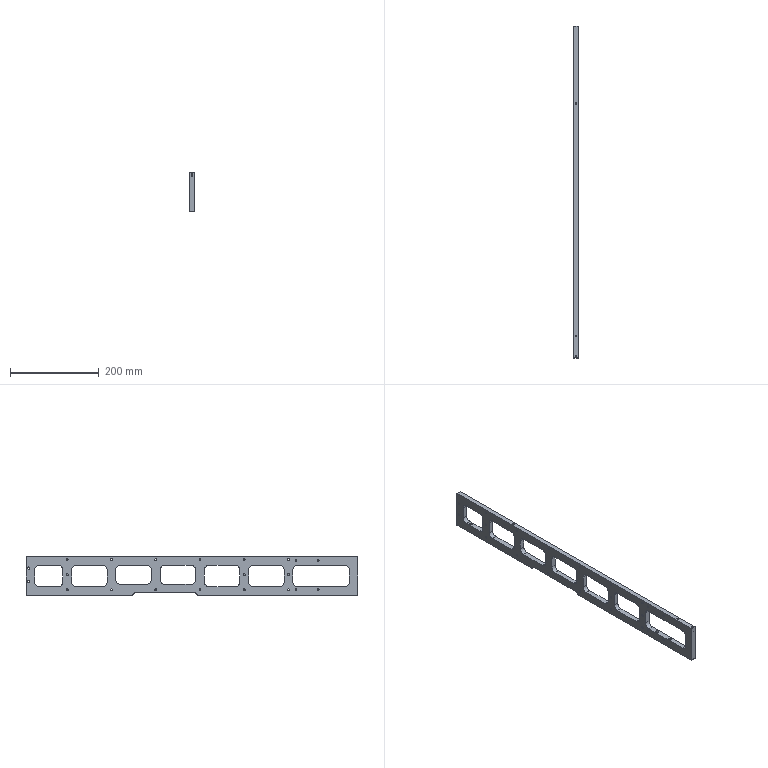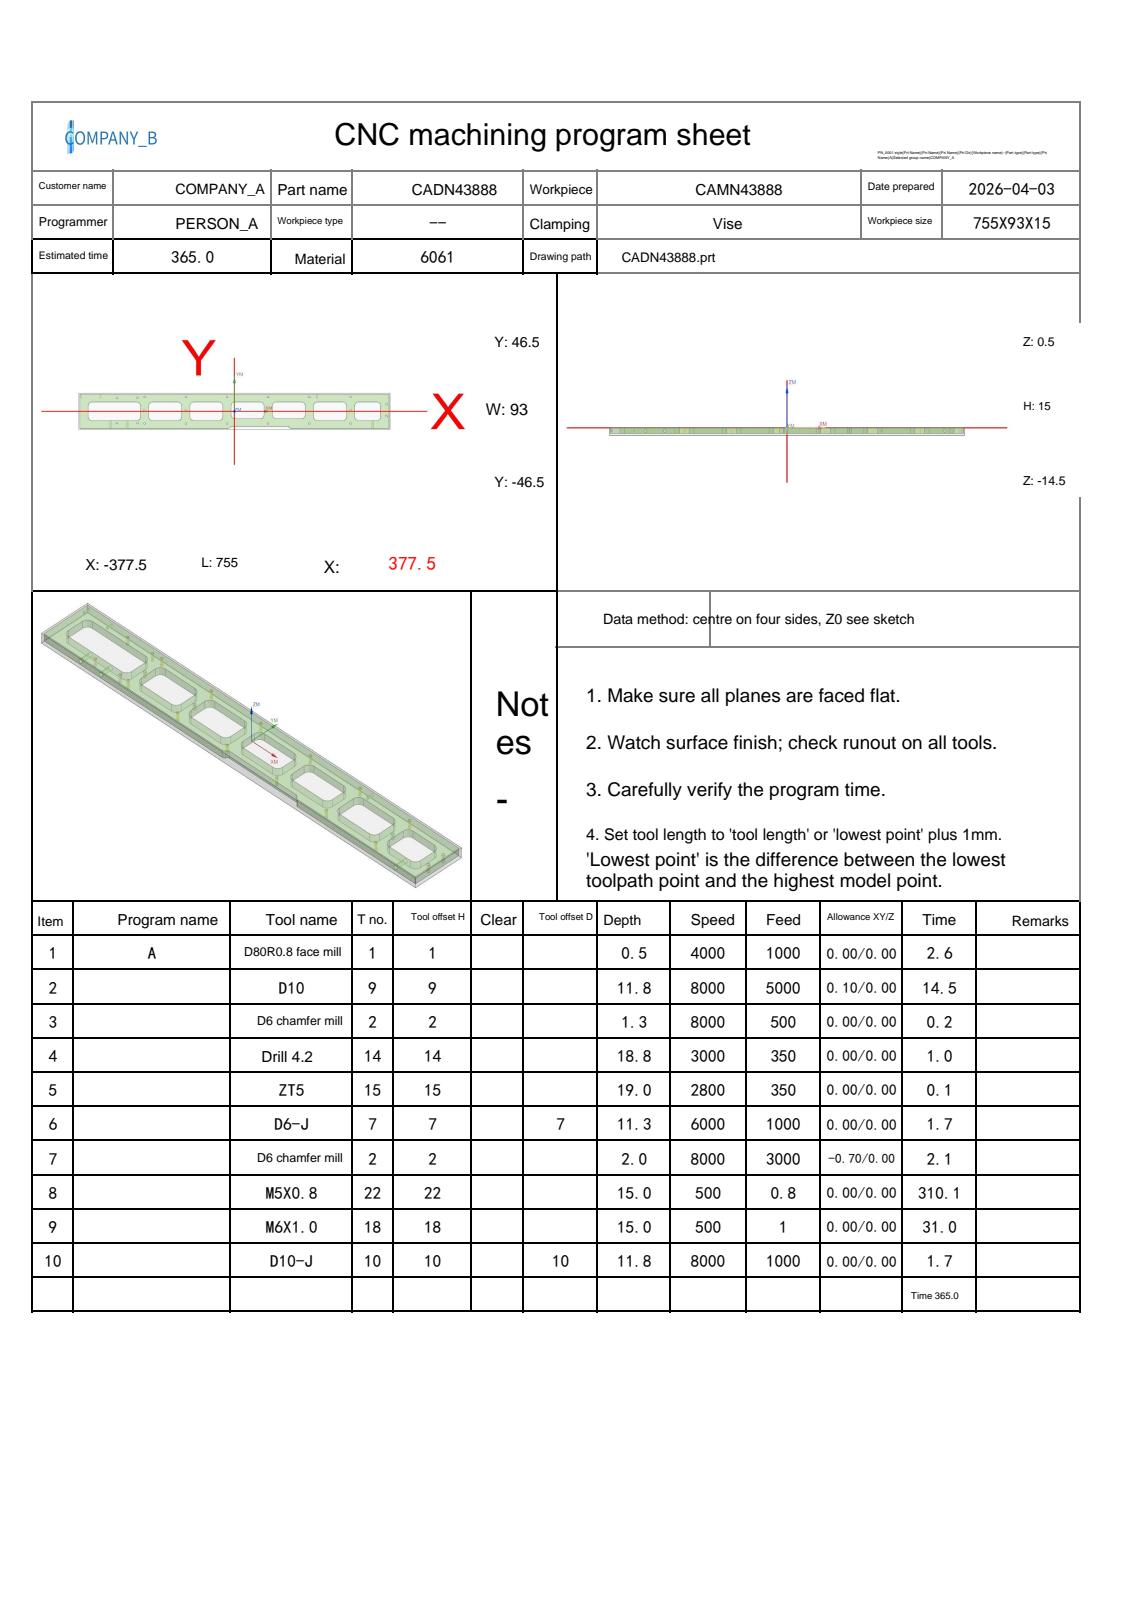NC program | NX | posted by the shop | part box 11 x 750 x 88 mm
Lines 1862 to 2351 of 2351:
N7 T02 M06
(D6 chamfer mill  D=6. R=0. H=02 ce=0.00 di=0.00)
G00 G90 G54 X-.25 Y45.828 M03 S8000
G43 H02 Z20.
M08
Z2.399
G01 Z-1.5 F3000.
G03 X-.33 Y45.528 I.52 J-.3
X-.03 Y45.008 I.6 J0.0
G01 X0.0 Y45.
X374.
G02 X376. Y43. I0.0 J-2.
G01 Y-43.
G02 X374. Y-45. I-2. J0.0
G01 X137.165
G02 X131.666 Y-41.4 I0.0 J6.
G03 X128. Y-39. I-3.666 J-1.6
G01 X-6.
G03 X-9.666 Y-41.4 I0.0 J-4.
G02 X-15.165 Y-45. I-5.499 J2.4
G01 X-374.
G02 X-376. Y-43. I0.0 J2.
G01 Y43.
G02 X-374. Y45. I2. J0.0
G01 X0.0
X.03 Y45.008
G03 X.33 Y45.528 I-.3 J.52
X.25 Y45.828 I-.6 J0.0
G01 Z2.399
G00 Z20.
X323.25 Y-22.172
Z2.399
G01 Z-1.5
G03 X323.17 Y-22.472 I.52 J-.3
X323.47 Y-22.992 I.6 J0.0
G01 X323.5 Y-23.
X345.
G03 X354. Y-14. I0.0 J9.
G01 Y14.
G03 X345. Y23. I-9. J0.0
G01 X302.
G03 X293. Y14. I0.0 J-9.
G01 Y-14.
G03 X302. Y-23. I9. J0.0
G01 X323.5
X323.53 Y-22.992
G03 X323.83 Y-22.472 I-.3 J.52
X323.75 Y-22.172 I-.6 J0.0
G01 Z2.399
G00 Z20.
X231.75
Z2.399
G01 Z-1.5
G03 X231.67 Y-22.472 I.52 J-.3
X231.97 Y-22.992 I.6 J0.0
G01 X232. Y-23.
X262.
G03 X271. Y-14. I0.0 J9.
G01 Y14.
G03 X262. Y23. I-9. J0.0
G01 X202.
G03 X193. Y14. I0.0 J-9.
G01 Y-14.
G03 X202. Y-23. I9. J0.0
G01 X232.
X232.03 Y-22.992
G03 X232.33 Y-22.472 I-.3 J.52
X232.25 Y-22.172 I-.6 J0.0
G01 Z2.399
G00 Z20.
X131.75 Y-17.172
Z2.399
G01 Z-1.5
G03 X131.67 Y-17.472 I.52 J-.3
X131.97 Y-17.992 I.6 J0.0
G01 X132. Y-18.
X162.
G03 X171. Y-9. I0.0 J9.
G01 Y14.
G03 X162. Y23. I-9. J0.0
G01 X102.
G03 X93. Y14. I0.0 J-9.
G01 Y-9.
G03 X102. Y-18. I9. J0.0
G01 X132.
X132.03 Y-17.992
G03 X132.33 Y-17.472 I-.3 J.52
X132.25 Y-17.172 I-.6 J0.0
G01 Z2.399
G00 Z20.
X31.75
Z2.399
G01 Z-1.5
G03 X31.67 Y-17.472 I.52 J-.3
X31.97 Y-17.992 I.6 J0.0
G01 X32. Y-18.
X62.
G03 X71. Y-9. I0.0 J9.
G01 Y14.
G03 X62. Y23. I-9. J0.0
G01 X2.
G03 X-7. Y14. I0.0 J-9.
G01 Y-9.
G03 X2. Y-18. I9. J0.0
G01 X32.
X32.03 Y-17.992
G03 X32.33 Y-17.472 I-.3 J.52
X32.25 Y-17.172 I-.6 J0.0
G01 Z2.399
G00 Z20.
X-68.25 Y-22.172
Z2.399
G01 Z-1.5
G03 X-68.33 Y-22.472 I.52 J-.3
X-68.03 Y-22.992 I.6 J0.0
G01 X-68. Y-23.
X-38.
G03 X-29. Y-14. I0.0 J9.
G01 Y14.
G03 X-38. Y23. I-9. J0.0
G01 X-98.
G03 X-107. Y14. I0.0 J-9.
G01 Y-14.
G03 X-98. Y-23. I9. J0.0
G01 X-68.
X-67.97 Y-22.992
G03 X-67.67 Y-22.472 I-.3 J.52
X-67.75 Y-22.172 I-.6 J0.0
G01 Z2.399
G00 Z20.
X-168.25
Z2.399
G01 Z-1.5
G03 X-168.33 Y-22.472 I.52 J-.3
X-168.03 Y-22.992 I.6 J0.0
G01 X-168. Y-23.
X-138.
G03 X-129. Y-14. I0.0 J9.
G01 Y14.
G03 X-138. Y23. I-9. J0.0
G01 X-198.
G03 X-207. Y14. I0.0 J-9.
G01 Y-14.
G03 X-198. Y-23. I9. J0.0
G01 X-168.
X-167.97 Y-22.992
G03 X-167.67 Y-22.472 I-.3 J.52
X-167.75 Y-22.172 I-.6 J0.0
G01 Z2.399
G00 Z20.
X-291.75
Z2.399
G01 Z-1.5
G03 X-291.83 Y-22.472 I.52 J-.3
X-291.53 Y-22.992 I.6 J0.0
G01 X-291.5 Y-23.
X-238.
G03 X-229. Y-14. I0.0 J9.
G01 Y14.
G03 X-238. Y23. I-9. J0.0
G01 X-345.
G03 X-354. Y14. I0.0 J-9.
G01 Y-14.
G03 X-345. Y-23. I9. J0.0
G01 X-291.5
X-291.47 Y-22.992
G03 X-291.17 Y-22.472 I-.3 J.52
X-291.25 Y-22.172 I-.6 J0.0
G01 Z2.399
G00 Z20.
G00 G90 X282.694 Y37.093 M03 S8000
Z20.
Z-.5
G01 Z-1. F500.
X283.5 Y37.2
G03 X282. Y38.7 I-1.5 J0.0
X280.3 Y37. I0.0 J-1.7
X282. Y35.3 I1.7 J0.0
X283.7 Y37. I0.0 J1.7
X282. Y38.7 I-1.7 J0.0
X280.5 Y37.2 I0.0 J-1.5
G01 X281.306 Y37.093
Z-.5
G00 Z20.
X282.694 Y-30.907
Z-.5
G01 Z-1.
X283.5 Y-30.8
G03 X282. Y-29.3 I-1.5 J0.0
X280.3 Y-31. I0.0 J-1.7
X282. Y-32.7 I1.7 J0.0
X283.7 Y-31. I0.0 J1.7
X282. Y-29.3 I-1.7 J0.0
X280.5 Y-30.8 I0.0 J-1.5
G01 X281.306 Y-30.907
Z-.5
G00 Z20.
X182.694
Z-.5
G01 Z-1.
X183.5 Y-30.8
G03 X182. Y-29.3 I-1.5 J0.0
X180.3 Y-31. I0.0 J-1.7
X182. Y-32.7 I1.7 J0.0
X183.7 Y-31. I0.0 J1.7
X182. Y-29.3 I-1.7 J0.0
X180.5 Y-30.8 I0.0 J-1.5
G01 X181.306 Y-30.907
Z-.5
G00 Z20.
X182.694 Y37.093
Z-.5
G01 Z-1.
X183.5 Y37.2
G03 X182. Y38.7 I-1.5 J0.0
X180.3 Y37. I0.0 J-1.7
X182. Y35.3 I1.7 J0.0
X183.7 Y37. I0.0 J1.7
X182. Y38.7 I-1.7 J0.0
X180.5 Y37.2 I0.0 J-1.5
G01 X181.306 Y37.093
Z-.5
G00 Z20.
X82.694
Z-.5
G01 Z-1.
X83.5 Y37.2
G03 X82. Y38.7 I-1.5 J0.0
X80.3 Y37. I0.0 J-1.7
X82. Y35.3 I1.7 J0.0
X83.7 Y37. I0.0 J1.7
X82. Y38.7 I-1.7 J0.0
X80.5 Y37.2 I0.0 J-1.5
G01 X81.306 Y37.093
Z-.5
G00 Z20.
X82.694 Y-30.907
Z-.5
G01 Z-1.
X83.5 Y-30.8
G03 X82. Y-29.3 I-1.5 J0.0
X80.3 Y-31. I0.0 J-1.7
X82. Y-32.7 I1.7 J0.0
X83.7 Y-31. I0.0 J1.7
X82. Y-29.3 I-1.7 J0.0
X80.5 Y-30.8 I0.0 J-1.5
G01 X81.306 Y-30.907
Z-.5
G00 Z20.
X-17.306
Z-.5
G01 Z-1.
X-16.5 Y-30.8
G03 X-18. Y-29.3 I-1.5 J0.0
X-19.7 Y-31. I0.0 J-1.7
X-18. Y-32.7 I1.7 J0.0
X-16.3 Y-31. I0.0 J1.7
X-18. Y-29.3 I-1.7 J0.0
X-19.5 Y-30.8 I0.0 J-1.5
G01 X-18.694 Y-30.907
Z-.5
G00 Z20.
X-17.306 Y37.093
Z-.5
G01 Z-1.
X-16.5 Y37.2
G03 X-18. Y38.7 I-1.5 J0.0
X-19.7 Y37. I0.0 J-1.7
X-18. Y35.3 I1.7 J0.0
X-16.3 Y37. I0.0 J1.7
X-18. Y38.7 I-1.7 J0.0
X-19.5 Y37.2 I0.0 J-1.5
G01 X-18.694 Y37.093
Z-.5
G00 Z20.
X-117.306
Z-.5
G01 Z-1.
X-116.5 Y37.2
G03 X-118. Y38.7 I-1.5 J0.0
X-119.7 Y37. I0.0 J-1.7
X-118. Y35.3 I1.7 J0.0
X-116.3 Y37. I0.0 J1.7
X-118. Y38.7 I-1.7 J0.0
X-119.5 Y37.2 I0.0 J-1.5
G01 X-118.694 Y37.093
Z-.5
G00 Z20.
X-117.306 Y-30.907
Z-.5
G01 Z-1.
X-116.5 Y-30.8
G03 X-118. Y-29.3 I-1.5 J0.0
X-119.7 Y-31. I0.0 J-1.7
X-118. Y-32.7 I1.7 J0.0
X-116.3 Y-31. I0.0 J1.7
X-118. Y-29.3 I-1.7 J0.0
X-119.5 Y-30.8 I0.0 J-1.5
G01 X-118.694 Y-30.907
Z-.5
G00 Z20.
X-217.306
Z-.5
G01 Z-1.
X-216.5 Y-30.8
G03 X-218. Y-29.3 I-1.5 J0.0
X-219.7 Y-31. I0.0 J-1.7
X-218. Y-32.7 I1.7 J0.0
X-216.3 Y-31. I0.0 J1.7
X-218. Y-29.3 I-1.7 J0.0
X-219.5 Y-30.8 I0.0 J-1.5
G01 X-218.694 Y-30.907
Z-.5
G00 Z20.
X-234.306 Y-30.157
Z-.5
G01 Z-1.
X-233.5 Y-30.05
G03 X-235. Y-28.55 I-1.5 J0.0
X-236.7 Y-30.25 I0.0 J-1.7
X-235. Y-31.95 I1.7 J0.0
X-233.3 Y-30.25 I0.0 J1.7
X-235. Y-28.55 I-1.7 J0.0
X-236.5 Y-30.05 I0.0 J-1.5
G01 X-235.694 Y-30.157
Z-.5
G00 Z20.
X-284.306
Z-.5
G01 Z-1.
X-283.5 Y-30.05
G03 X-285. Y-28.55 I-1.5 J0.0
X-286.7 Y-30.25 I0.0 J-1.7
X-285. Y-31.95 I1.7 J0.0
X-283.3 Y-30.25 I0.0 J1.7
X-285. Y-28.55 I-1.7 J0.0
X-286.5 Y-30.05 I0.0 J-1.5
G01 X-285.694 Y-30.157
Z-.5
G00 Z20.
X-284.306 Y35.343
Z-.5
G01 Z-1.
X-283.5 Y35.45
G03 X-285. Y36.95 I-1.5 J0.0
X-286.7 Y35.25 I0.0 J-1.7
X-285. Y33.55 I1.7 J0.0
X-283.3 Y35.25 I0.0 J1.7
X-285. Y36.95 I-1.7 J0.0
X-286.5 Y35.45 I0.0 J-1.5
G01 X-285.694 Y35.343
Z-.5
G00 Z20.
X-234.306
Z-.5
G01 Z-1.
X-233.5 Y35.45
G03 X-235. Y36.95 I-1.5 J0.0
X-236.7 Y35.25 I0.0 J-1.7
X-235. Y33.55 I1.7 J0.0
X-233.3 Y35.25 I0.0 J1.7
X-235. Y36.95 I-1.7 J0.0
X-236.5 Y35.45 I0.0 J-1.5
G01 X-235.694 Y35.343
Z-.5
G00 Z20.
X-217.306 Y37.093
Z-.5
G01 Z-1.
X-216.5 Y37.2
G03 X-218. Y38.7 I-1.5 J0.0
X-219.7 Y37. I0.0 J-1.7
X-218. Y35.3 I1.7 J0.0
X-216.3 Y37. I0.0 J1.7
X-218. Y38.7 I-1.7 J0.0
X-219.5 Y37.2 I0.0 J-1.5
G01 X-218.694 Y37.093
Z-.5
G00 Z20.
G00 G90 X370.028 Y-11.58 M03 S8000
Z20.
Z-.6
G01 Z-1.1 F500.
X370.5 Y-11.388
G03 X369. Y-9.888 I-1.5 J0.0
X366.89 Y-11.998 I0.0 J-2.11
X369. Y-14.108 I2.11 J0.0
X371.11 Y-11.998 I0.0 J2.11
X369. Y-9.888 I-2.11 J0.0
X367.5 Y-11.388 I0.0 J-1.5
G01 X367.972 Y-11.58
Z-.6
G00 Z20.
X370.028 Y18.42
Z-.6
G01 Z-1.1
X370.5 Y18.612
G03 X369. Y20.112 I-1.5 J0.0
X366.89 Y18.002 I0.0 J-2.11
X369. Y15.892 I2.11 J0.0
X371.11 Y18.002 I0.0 J2.11
X369. Y20.112 I-2.11 J0.0
X367.5 Y18.612 I0.0 J-1.5
G01 X367.972 Y18.42
Z-.6
G00 Z20.
G91 G28 Z0.0
M05
M09
G91 G28 Z0.0
M01
N8 T22 M06
(M5X0.8 D=4.2 DR_a=180 H=22)
G00 G90 G54 X282. Y-31. M03 S500
G43 H22 Z20.
M08
G95
G98 G84 X282. Y-31. Z-14.5 R1. F.8 Q3.
Y37.
X182.
Y-31.
X82.
Y37.
X-18.
Y-31.
X-118.
Y37.
X-218.
X-235. Y35.25
X-285.
Y-30.25
X-235.
X-218. Y-31.
G80
G94
G00 Z20.
G91 G28 Z0.0
M05
M09
G91 G28 Z0.0
M01
N9 T18 M06
(M6X1.0 D=5. DR_a=180 H=18)
G00 G90 G54 X369. Y-11.998 M03 S500
G43 H18 Z20.
M08
G95
G98 G84 X369. Y-11.998 Z-14.5 R1. F1. Q3.
Y18.002
G80
G94
G00 Z20.
G91 G28 Z0.0
M05
M09
G91 G28 Z0.0
M01
N10 T10 M06
(D10-J  D=10. R=0. H=10 ce=0.00 di=0.00)
G00 G90 G54 X-375.012 Y50.128 M03 S8000
G43 H10 Z20.
M08
Z-10.8
G01 Z-11.3 F1000.
G41 D10
X-374.997 Y49.929
G03 X-374. Y49. I.997 J.071
G01 X374.
G02 X380. Y43. I0.0 J-6.
G01 Y-43.
G02 X374. Y-49. I-6. J0.0
G01 X137.165
G02 X128. Y-43. I0.0 J10.
G01 X-6.
G02 X-15.165 Y-49. I-9.165 J4.
G01 X-374.
G02 X-380. Y-43. I0.0 J6.
G01 Y43.
G02 X-374. Y49. I6. J0.0
G01 X-373.5
G03 X-372.5 Y50. I0.0 J1.
G01 G40 Y50.2
Z-10.8
G00 Z20.
M05
M09
G91 G28 Z0.0
G91 G28 Y0.0
M30
%